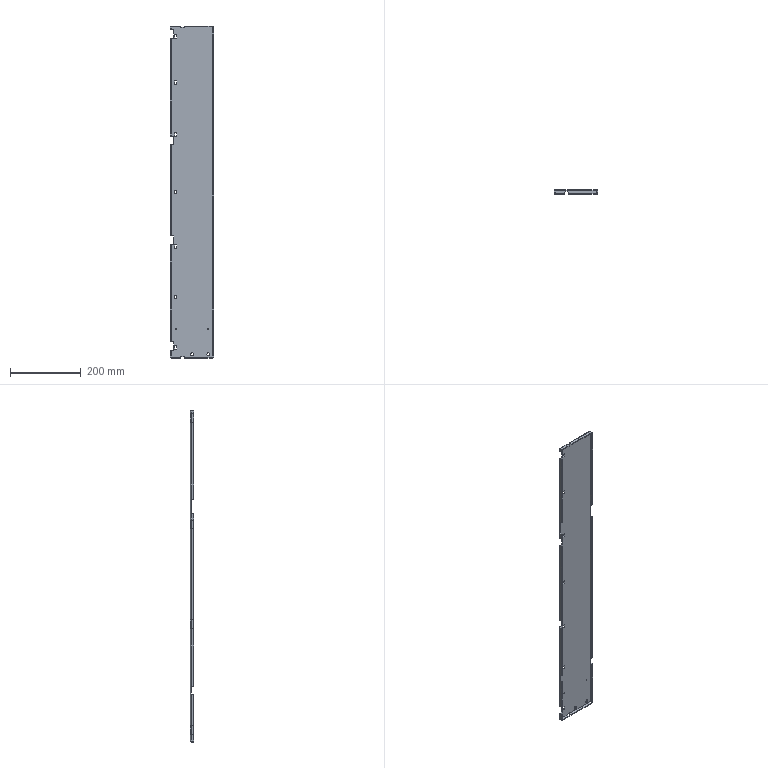Part | NX | features solid 2 | 1 solid | 168 faces | box 124 x 10 x 941 mm | volume 319730 mm3 | plane 150 | cylinder 18 | commonest cylinder face diameters 5 x10 3.2 x4 8.3 x4